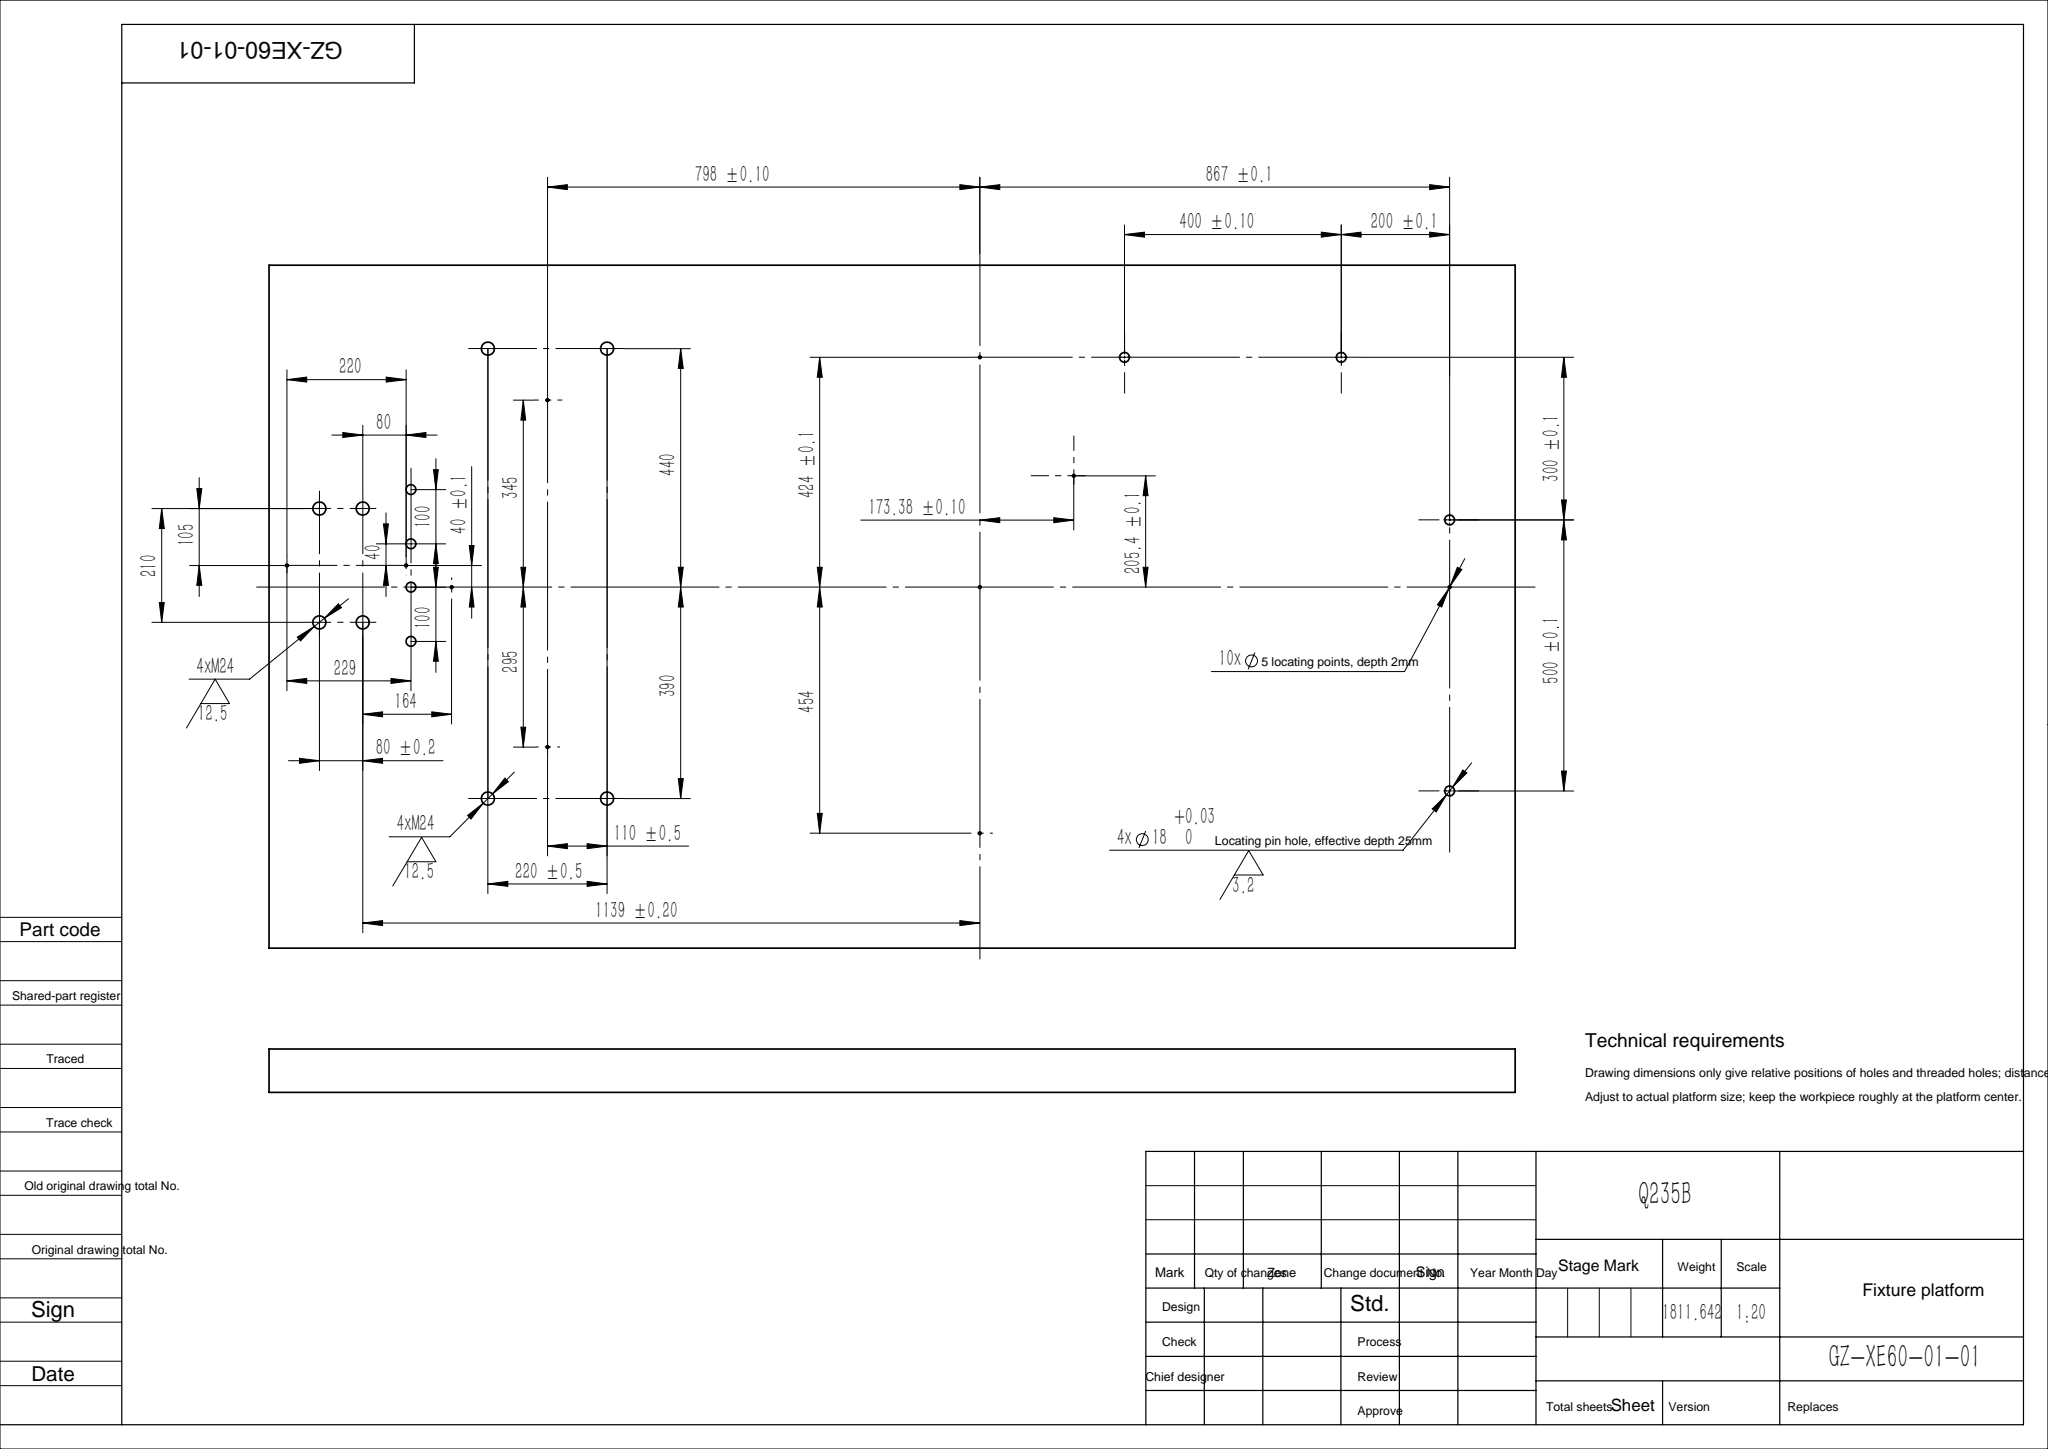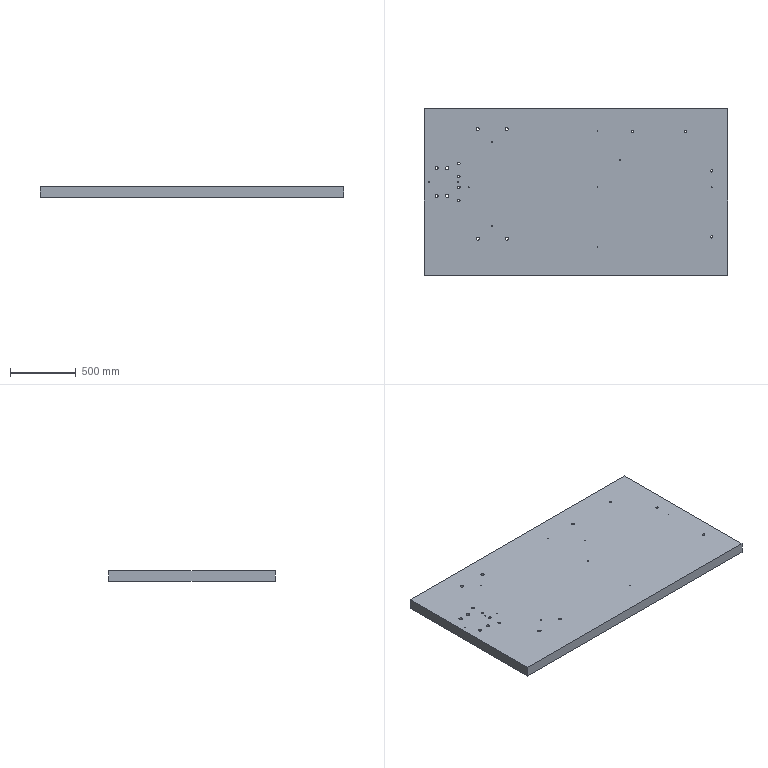Part | SolidWorks | features Extrusion 1 | 1 solid | 58 faces | box 2300 x 1260 x 80 mm | volume 231371903 mm3 | cylinder 52 | plane 6 | commonest cylinder face diameters 5 x20 18 x16 24 x16